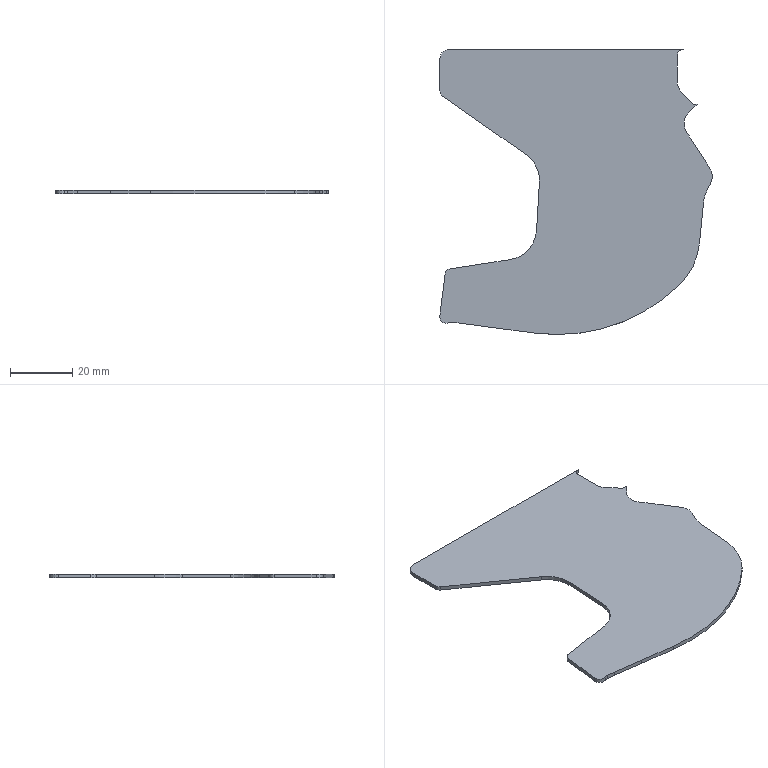Part | STEP file | gslz 2016.10.28-13_id218_x_t | 1 solid | 34 faces | box 87.403 x 91.412 x 1.25 mm | volume 7185 mm3 | plane 19 | cylinder 15 | commonest cylinder face diameters 4 x6 10 x3 20 x3 6 x1 44 x1 112.702 x1